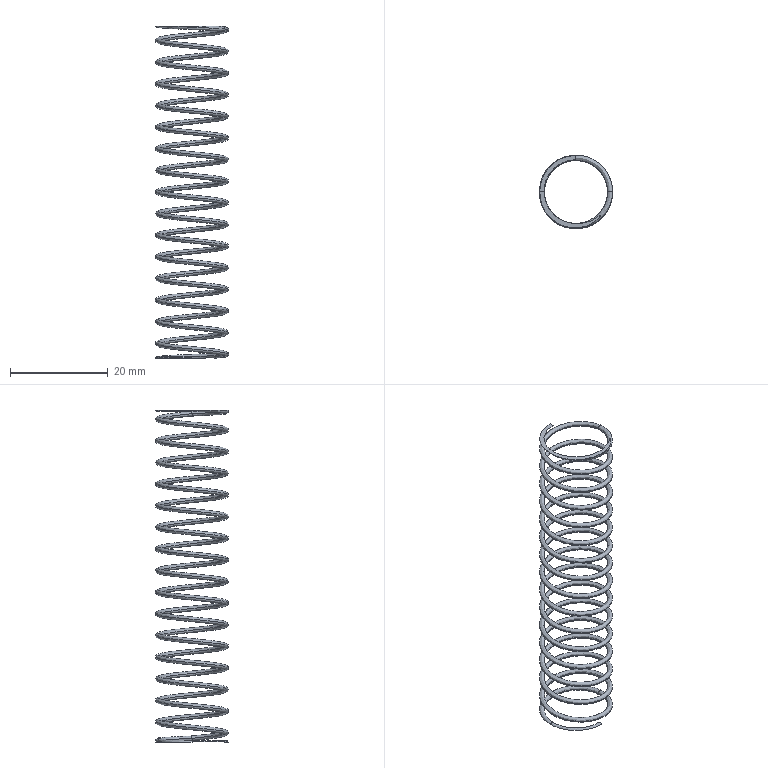Part | STEP file | X77B-01005 | 1 solid | 12 faces | box 15 x 15 x 68 mm | volume 612.5 mm3 | spline 8 | plane 4